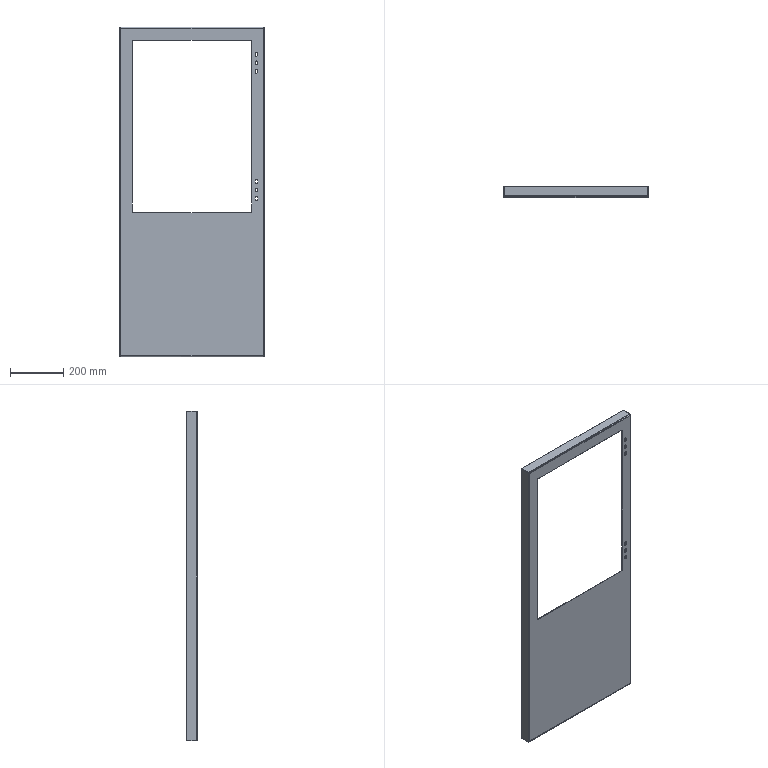Part | SolidWorks | features ICE 2, EdgeFlange 1, FlatPattern 1, SMBaseFlange 1, SheetMetal 1 | 1 solid | 76 faces | box 546 x 40 x 1245 mm | volume 1034914 mm3 | plane 38 | cylinder 30 | spline 8 | commonest cylinder face diameters 9 x18 4 x8 8 x4